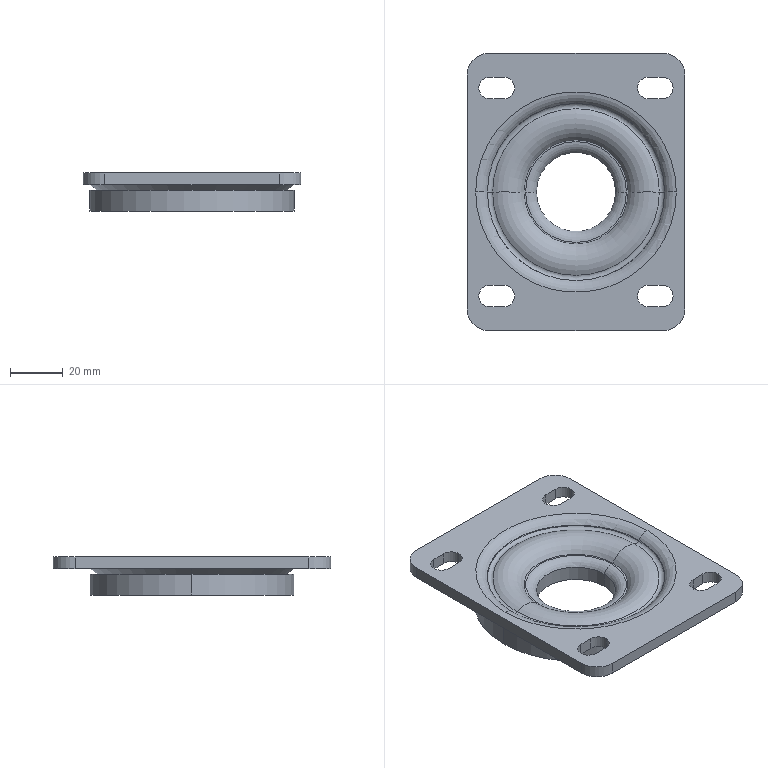Part | SolidWorks | features BaseBody 4, CombineBodies 2, ICE 2, MoveCopyBody 1, MoveFace 1, Scale 1 | 1 solid | 49 faces | box 82.5 x 105 x 14.438 mm | volume 61756 mm3 | cylinder 20 | plane 17 | torus 8 | cone 4 | commonest cylinder face diameters 8.25 x12 16.5 x4 30 x2 77.25 x2
STEP:
#1=CARTESIAN_POINT('',(-15.004,56.345,110.911));
#2=VERTEX_POINT('',#1);
#3=CARTESIAN_POINT('',(14.996,56.345,110.911));
#4=VERTEX_POINT('',#3);
#5=CARTESIAN_POINT('',(-0.004235,56.345,110.911));
#6=DIRECTION('',(0.,0.,1.));
#7=DIRECTION('',(-1.,0.,0.));
#8=AXIS2_PLACEMENT_3D('',#5,#6,#7);
#9=CIRCLE('',#8,15.);
#10=EDGE_CURVE('',#2,#4,#9,.T.);
#11=ORIENTED_EDGE('',*,*,#10,.T.);
#12=CARTESIAN_POINT('',(14.996,56.345,105.247));
#13=VERTEX_POINT('',#12);
#14=CARTESIAN_POINT('',(14.996,56.345,119.684));
#15=DIRECTION('',(0.,0.,-1.));
#16=VECTOR('',#15,1000.);
#17=LINE('',#14,#16);
#18=EDGE_CURVE('',#4,#13,#17,.T.);
#19=ORIENTED_EDGE('',*,*,#18,.T.);
#20=CARTESIAN_POINT('',(-15.004,56.345,105.247));
#21=VERTEX_POINT('',#20);
#22=CARTESIAN_POINT('',(-0.004235,56.345,105.247));
#23=DIRECTION('',(0.,0.,-1.));
#24=DIRECTION('',(-1.,0.,0.));
#25=AXIS2_PLACEMENT_3D('',#22,#23,#24);
#26=CIRCLE('',#25,15.);
#27=EDGE_CURVE('',#13,#21,#26,.T.);
#28=ORIENTED_EDGE('',*,*,#27,.T.);
#29=CARTESIAN_POINT('',(-15.004,56.345,119.684));
#30=DIRECTION('',(0.,0.,-1.));
#31=VECTOR('',#30,1000.);
#32=LINE('',#29,#31);
#33=EDGE_CURVE('',#2,#21,#32,.T.);
#34=ORIENTED_EDGE('',*,*,#33,.F.);
#35=EDGE_LOOP('',(#11,#19,#28,#34));
#36=FACE_OUTER_BOUND('',#35,.T.);
#37=CARTESIAN_POINT('',(-0.004235,56.345,119.684));
#38=DIRECTION('',(0.,0.,-1.));
#39=DIRECTION('',(-1.,0.,0.));
#40=AXIS2_PLACEMENT_3D('',#37,#38,#39);
#41=CYLINDRICAL_SURFACE('',#40,15.);
#42=ADVANCED_FACE('',(#36),#41,.F.);
#43=CARTESIAN_POINT('',(-0.004235,56.345,110.911));
#44=DIRECTION('',(0.,0.,1.));
#45=DIRECTION('',(-1.,0.,0.));
#46=AXIS2_PLACEMENT_3D('',#43,#44,#45);
#47=CIRCLE('',#46,15.);
#48=EDGE_CURVE('',#4,#2,#47,.T.);
#49=ORIENTED_EDGE('',*,*,#48,.F.);
#50=CARTESIAN_POINT('',(19.068,56.345,113.497));
#51=VERTEX_POINT('',#50);
#52=CARTESIAN_POINT('',(19.068,56.345,108.997));
#53=DIRECTION('',(0.,-1.,0.));
#54=DIRECTION('',(0.,0.,-1.));
#55=AXIS2_PLACEMENT_3D('',#52,#53,#54);
#56=CIRCLE('',#55,4.5);
#57=EDGE_CURVE('',#51,#4,#56,.T.);
#58=ORIENTED_EDGE('',*,*,#57,.F.);
#59=CARTESIAN_POINT('',(-19.077,56.345,113.497));
#60=VERTEX_POINT('',#59);
#61=CARTESIAN_POINT('',(-0.004235,56.345,113.497));
#62=DIRECTION('',(0.,0.,1.));
#63=DIRECTION('',(1.,0.,0.));
#64=AXIS2_PLACEMENT_3D('',#61,#62,#63);
#65=CIRCLE('',#64,19.072);
#66=EDGE_CURVE('',#51,#60,#65,.T.);
#67=ORIENTED_EDGE('',*,*,#66,.T.);
#68=CARTESIAN_POINT('',(-19.077,56.345,108.997));
#69=DIRECTION('',(0.,1.,0.));
#70=DIRECTION('',(-1.,0.,0.));
#71=AXIS2_PLACEMENT_3D('',#68,#69,#70);
#72=CIRCLE('',#71,4.5);
#73=EDGE_CURVE('',#60,#2,#72,.T.);
#74=ORIENTED_EDGE('',*,*,#73,.T.);
#75=EDGE_LOOP('',(#49,#58,#67,#74));
#76=FACE_OUTER_BOUND('',#75,.T.);
#77=CARTESIAN_POINT('',(-0.004235,56.345,108.997));
#78=DIRECTION('',(0.,0.,1.));
#79=DIRECTION('',(1.,0.,0.));
#80=AXIS2_PLACEMENT_3D('',#77,#78,#79);
#81=TOROIDAL_SURFACE('',#80,19.072,4.5);
#82=ADVANCED_FACE('',(#76),#81,.T.);
#83=CARTESIAN_POINT('',(31.504,56.345,116.515));
#84=VERTEX_POINT('',#83);
#85=CARTESIAN_POINT('',(-31.512,56.345,116.515));
#86=VERTEX_POINT('',#85);
#87=CARTESIAN_POINT('',(-0.004235,56.345,116.515));
#88=DIRECTION('',(0.,0.,1.));
#89=DIRECTION('',(1.,0.,0.));
#90=AXIS2_PLACEMENT_3D('',#87,#88,#89);
#91=CIRCLE('',#90,31.508);
#92=EDGE_CURVE('',#84,#86,#91,.T.);
#93=ORIENTED_EDGE('',*,*,#92,.T.);
#94=CARTESIAN_POINT('',(-19.74,56.345,113.497));
#95=VERTEX_POINT('',#94);
#96=CARTESIAN_POINT('',(-27.146,56.345,109.077));
#97=DIRECTION('',(0.,1.,0.));
#98=DIRECTION('',(-1.,0.,0.));
#99=AXIS2_PLACEMENT_3D('',#96,#97,#98);
#100=CIRCLE('',#99,8.625);
#101=EDGE_CURVE('',#86,#95,#100,.T.);
#102=ORIENTED_EDGE('',*,*,#101,.T.);
#103=CARTESIAN_POINT('',(19.732,56.345,113.497));
#104=VERTEX_POINT('',#103);
#105=CARTESIAN_POINT('',(-0.004235,56.345,113.497));
#106=DIRECTION('',(0.,0.,1.));
#107=DIRECTION('',(1.,0.,0.));
#108=AXIS2_PLACEMENT_3D('',#105,#106,#107);
#109=CIRCLE('',#108,19.736);
#110=EDGE_CURVE('',#104,#95,#109,.T.);
#111=ORIENTED_EDGE('',*,*,#110,.F.);
#112=CARTESIAN_POINT('',(27.138,56.345,109.077));
#113=DIRECTION('',(0.,-1.,0.));
#114=DIRECTION('',(0.,0.,-1.));
#115=AXIS2_PLACEMENT_3D('',#112,#113,#114);
#116=CIRCLE('',#115,8.625);
#117=EDGE_CURVE('',#84,#104,#116,.T.);
#118=ORIENTED_EDGE('',*,*,#117,.F.);
#119=EDGE_LOOP('',(#93,#102,#111,#118));
#120=FACE_OUTER_BOUND('',#119,.T.);
#121=CARTESIAN_POINT('',(-0.004235,56.345,109.077));
#122=DIRECTION('',(0.,0.,1.));
#123=DIRECTION('',(1.,0.,0.));
#124=AXIS2_PLACEMENT_3D('',#121,#122,#123);
#125=TOROIDAL_SURFACE('',#124,27.142,8.625);
#126=ADVANCED_FACE('',(#120),#125,.T.);
#127=CARTESIAN_POINT('',(-0.004235,56.345,116.515));
#128=DIRECTION('',(0.,0.,1.));
#129=DIRECTION('',(1.,0.,0.));
#130=AXIS2_PLACEMENT_3D('',#127,#128,#129);
#131=CIRCLE('',#130,31.508);
#132=EDGE_CURVE('',#86,#84,#131,.T.);
#133=ORIENTED_EDGE('',*,*,#132,.F.);
#134=CARTESIAN_POINT('',(-33.528,56.345,117.013));
#135=VERTEX_POINT('',#134);
#136=CARTESIAN_POINT('',(-32.261,56.345,117.815));
#137=DIRECTION('',(0.,1.,0.));
#138=DIRECTION('',(-1.,0.,0.));
#139=AXIS2_PLACEMENT_3D('',#136,#137,#138);
#140=CIRCLE('',#139,1.5);
#141=EDGE_CURVE('',#86,#135,#140,.T.);
#142=ORIENTED_EDGE('',*,*,#141,.T.);
#143=CARTESIAN_POINT('',(33.52,56.345,117.013));
#144=VERTEX_POINT('',#143);
#145=CARTESIAN_POINT('',(-0.004235,56.345,117.013));
#146=DIRECTION('',(0.,0.,1.));
#147=DIRECTION('',(1.,0.,0.));
#148=AXIS2_PLACEMENT_3D('',#145,#146,#147);
#149=CIRCLE('',#148,33.524);
#150=EDGE_CURVE('',#135,#144,#149,.T.);
#151=ORIENTED_EDGE('',*,*,#150,.T.);
#152=CARTESIAN_POINT('',(32.252,56.345,117.815));
#153=DIRECTION('',(0.,-1.,0.));
#154=DIRECTION('',(0.,0.,-1.));
#155=AXIS2_PLACEMENT_3D('',#152,#153,#154);
#156=CIRCLE('',#155,1.5);
#157=EDGE_CURVE('',#84,#144,#156,.T.);
#158=ORIENTED_EDGE('',*,*,#157,.F.);
#159=EDGE_LOOP('',(#133,#142,#151,#158));
#160=FACE_OUTER_BOUND('',#159,.T.);
#161=CARTESIAN_POINT('',(-0.004235,56.345,117.815));
#162=DIRECTION('',(0.,0.,1.));
#163=DIRECTION('',(1.,0.,0.));
#164=AXIS2_PLACEMENT_3D('',#161,#162,#163);
#165=TOROIDAL_SURFACE('',#164,32.256,1.5);
#166=ADVANCED_FACE('',(#160),#165,.F.);
#167=ORIENTED_EDGE('',*,*,#150,.F.);
#168=CARTESIAN_POINT('',(-33.673,56.345,117.242));
#169=VERTEX_POINT('',#168);
#170=CARTESIAN_POINT('',(-33.673,56.345,117.242));
#171=DIRECTION('',(-0.5345,0.,0.8452));
#172=VECTOR('',#171,1000.);
#173=LINE('',#170,#172);
#174=EDGE_CURVE('',#135,#169,#173,.T.);
#175=ORIENTED_EDGE('',*,*,#174,.T.);
#176=CARTESIAN_POINT('',(33.665,56.345,117.242));
#177=VERTEX_POINT('',#176);
#178=CARTESIAN_POINT('',(-0.004235,56.345,117.242));
#179=DIRECTION('',(0.,0.,1.));
#180=DIRECTION('',(1.,0.,0.));
#181=AXIS2_PLACEMENT_3D('',#178,#179,#180);
#182=CIRCLE('',#181,33.669);
#183=EDGE_CURVE('',#169,#177,#182,.T.);
#184=ORIENTED_EDGE('',*,*,#183,.T.);
#185=CARTESIAN_POINT('',(33.665,56.345,117.242));
#186=DIRECTION('',(0.5345,0.,0.8452));
#187=VECTOR('',#186,1000.);
#188=LINE('',#185,#187);
#189=EDGE_CURVE('',#144,#177,#188,.T.);
#190=ORIENTED_EDGE('',*,*,#189,.F.);
#191=EDGE_LOOP('',(#167,#175,#184,#190));
#192=FACE_OUTER_BOUND('',#191,.T.);
#193=CARTESIAN_POINT('',(-0.004235,56.345,117.242));
#194=DIRECTION('',(0.,0.,1.));
#195=DIRECTION('',(1.,0.,0.));
#196=AXIS2_PLACEMENT_3D('',#193,#194,#195);
#197=CONICAL_SURFACE('',#196,33.669,0.5639);
#198=ADVANCED_FACE('',(#192),#197,.F.);
#199=CARTESIAN_POINT('',(-37.966,56.345,119.684));
#200=VERTEX_POINT('',#199);
#201=CARTESIAN_POINT('',(37.958,56.345,119.684));
#202=VERTEX_POINT('',#201);
#203=CARTESIAN_POINT('',(-0.004235,56.345,119.684));
#204=DIRECTION('',(0.,0.,-1.));
#205=DIRECTION('',(1.,0.,0.));
#206=AXIS2_PLACEMENT_3D('',#203,#204,#205);
#207=CIRCLE('',#206,37.962);
#208=EDGE_CURVE('',#200,#202,#207,.T.);
#209=ORIENTED_EDGE('',*,*,#208,.F.);
#210=CARTESIAN_POINT('',(-38.11,56.345,114.436));
#211=DIRECTION('',(0.,1.,0.));
#212=DIRECTION('',(-1.,0.,0.));
#213=AXIS2_PLACEMENT_3D('',#210,#211,#212);
#214=CIRCLE('',#213,5.25);
#215=EDGE_CURVE('',#200,#169,#214,.T.);
#216=ORIENTED_EDGE('',*,*,#215,.T.);
#217=CARTESIAN_POINT('',(-0.004235,56.345,117.242));
#218=DIRECTION('',(0.,0.,1.));
#219=DIRECTION('',(1.,0.,0.));
#220=AXIS2_PLACEMENT_3D('',#217,#218,#219);
#221=CIRCLE('',#220,33.669);
#222=EDGE_CURVE('',#177,#169,#221,.T.);
#223=ORIENTED_EDGE('',*,*,#222,.F.);
#224=CARTESIAN_POINT('',(38.102,56.345,114.436));
#225=DIRECTION('',(0.,-1.,0.));
#226=DIRECTION('',(0.,0.,-1.));
#227=AXIS2_PLACEMENT_3D('',#224,#225,#226);
#228=CIRCLE('',#227,5.25);
#229=EDGE_CURVE('',#202,#177,#228,.T.);
#230=ORIENTED_EDGE('',*,*,#229,.F.);
#231=EDGE_LOOP('',(#209,#216,#223,#230));
#232=FACE_OUTER_BOUND('',#231,.T.);
#233=CARTESIAN_POINT('',(-0.004235,56.345,114.436));
#234=DIRECTION('',(0.,0.,1.));
#235=DIRECTION('',(1.,0.,0.));
#236=AXIS2_PLACEMENT_3D('',#233,#234,#235);
#237=TOROIDAL_SURFACE('',#236,38.106,5.25);
#238=ADVANCED_FACE('',(#232),#237,.T.);
#239=CARTESIAN_POINT('',(38.621,56.345,105.247));
#240=VERTEX_POINT('',#239);
#241=CARTESIAN_POINT('',(-38.629,56.345,105.247));
#242=VERTEX_POINT('',#241);
#243=CARTESIAN_POINT('',(-0.004235,56.345,105.247));
#244=DIRECTION('',(0.,0.,1.));
#245=DIRECTION('',(1.,0.,0.));
#246=AXIS2_PLACEMENT_3D('',#243,#244,#245);
#247=CIRCLE('',#246,38.625);
#248=EDGE_CURVE('',#240,#242,#247,.T.);
#249=ORIENTED_EDGE('',*,*,#248,.T.);
#250=CARTESIAN_POINT('',(-38.629,56.345,113.122));
#251=VERTEX_POINT('',#250);
#252=CARTESIAN_POINT('',(-38.629,56.345,2.684));
#253=DIRECTION('',(0.,0.,1.));
#254=VECTOR('',#253,1000.);
#255=LINE('',#252,#254);
#256=EDGE_CURVE('',#242,#251,#255,.T.);
#257=ORIENTED_EDGE('',*,*,#256,.T.);
#258=CARTESIAN_POINT('',(38.621,56.345,113.122));
#259=VERTEX_POINT('',#258);
#260=CARTESIAN_POINT('',(-0.004235,56.345,113.122));
#261=DIRECTION('',(0.,0.,1.));
#262=DIRECTION('',(1.,0.,0.));
#263=AXIS2_PLACEMENT_3D('',#260,#261,#262);
#264=CIRCLE('',#263,38.625);
#265=EDGE_CURVE('',#259,#251,#264,.T.);
#266=ORIENTED_EDGE('',*,*,#265,.F.);
#267=CARTESIAN_POINT('',(38.621,56.345,2.684));
#268=DIRECTION('',(0.,0.,1.));
#269=VECTOR('',#268,1000.);
#270=LINE('',#267,#269);
#271=EDGE_CURVE('',#240,#259,#270,.T.);
#272=ORIENTED_EDGE('',*,*,#271,.F.);
#273=EDGE_LOOP('',(#249,#257,#266,#272));
#274=FACE_OUTER_BOUND('',#273,.T.);
#275=CARTESIAN_POINT('',(-0.004235,56.345,2.684));
#276=DIRECTION('',(0.,0.,1.));
#277=DIRECTION('',(1.,0.,0.));
#278=AXIS2_PLACEMENT_3D('',#275,#276,#277);
#279=CYLINDRICAL_SURFACE('',#278,38.625);
#280=ADVANCED_FACE('',(#274),#279,.T.);
#281=CARTESIAN_POINT('',(35.782,56.345,113.122));
#282=VERTEX_POINT('',#281);
#283=CARTESIAN_POINT('',(-35.79,56.345,113.122));
#284=VERTEX_POINT('',#283);
#285=CARTESIAN_POINT('',(-0.004235,56.345,113.122));
#286=DIRECTION('',(0.,0.,1.));
#287=DIRECTION('',(1.,0.,0.));
#288=AXIS2_PLACEMENT_3D('',#285,#286,#287);
#289=CIRCLE('',#288,35.786);
#290=EDGE_CURVE('',#282,#284,#289,.T.);
#291=ORIENTED_EDGE('',*,*,#290,.T.);
#292=CARTESIAN_POINT('',(-38.629,56.345,115.184));
#293=VERTEX_POINT('',#292);
#294=CARTESIAN_POINT('',(-38.629,56.345,115.184));
#295=DIRECTION('',(-0.809,0.,0.5878));
#296=VECTOR('',#295,1000.);
#297=LINE('',#294,#296);
#298=EDGE_CURVE('',#284,#293,#297,.T.);
#299=ORIENTED_EDGE('',*,*,#298,.T.);
#300=CARTESIAN_POINT('',(38.621,56.345,115.184));
#301=VERTEX_POINT('',#300);
#302=CARTESIAN_POINT('',(-0.004235,56.345,115.184));
#303=DIRECTION('',(0.,0.,-1.));
#304=DIRECTION('',(-1.,0.,0.));
#305=AXIS2_PLACEMENT_3D('',#302,#303,#304);
#306=CIRCLE('',#305,38.625);
#307=EDGE_CURVE('',#293,#301,#306,.T.);
#308=ORIENTED_EDGE('',*,*,#307,.T.);
#309=CARTESIAN_POINT('',(38.621,56.345,115.184));
#310=DIRECTION('',(0.809,0.,0.5878));
#311=VECTOR('',#310,1000.);
#312=LINE('',#309,#311);
#313=EDGE_CURVE('',#282,#301,#312,.T.);
#314=ORIENTED_EDGE('',*,*,#313,.F.);
#315=EDGE_LOOP('',(#291,#299,#308,#314));
#316=FACE_OUTER_BOUND('',#315,.T.);
#317=CARTESIAN_POINT('',(-0.004235,56.345,115.184));
#318=DIRECTION('',(0.,0.,1.));
#319=DIRECTION('',(1.,0.,0.));
#320=AXIS2_PLACEMENT_3D('',#317,#318,#319);
#321=CONICAL_SURFACE('',#320,38.625,0.9425);
#322=ADVANCED_FACE('',(#316),#321,.T.);
#323=CARTESIAN_POINT('',(-27.379,21.095,115.184));
#324=VERTEX_POINT('',#323);
#325=CARTESIAN_POINT('',(-23.254,16.97,115.184));
#326=VERTEX_POINT('',#325);
#327=CARTESIAN_POINT('',(-27.379,16.97,115.184));
#328=DIRECTION('',(0.,0.,-1.));
#329=DIRECTION('',(-1.,0.,0.));
#330=AXIS2_PLACEMENT_3D('',#327,#328,#329);
#331=CIRCLE('',#330,4.125);
#332=EDGE_CURVE('',#324,#326,#331,.T.);
#333=ORIENTED_EDGE('',*,*,#332,.T.);
#334=CARTESIAN_POINT('',(-23.254,16.97,119.684));
#335=VERTEX_POINT('',#334);
#336=CARTESIAN_POINT('',(-23.254,16.97,115.184));
#337=DIRECTION('',(0.,0.,1.));
#338=VECTOR('',#337,1000.);
#339=LINE('',#336,#338);
#340=EDGE_CURVE('',#326,#335,#339,.T.);
#341=ORIENTED_EDGE('',*,*,#340,.T.);
#342=CARTESIAN_POINT('',(-27.379,21.095,119.684));
#343=VERTEX_POINT('',#342);
#344=CARTESIAN_POINT('',(-27.379,16.97,119.684));
#345=DIRECTION('',(0.,0.,-1.));
#346=DIRECTION('',(-1.,0.,0.));
#347=AXIS2_PLACEMENT_3D('',#344,#345,#346);
#348=CIRCLE('',#347,4.125);
#349=EDGE_CURVE('',#343,#335,#348,.T.);
#350=ORIENTED_EDGE('',*,*,#349,.F.);
#351=CARTESIAN_POINT('',(-27.379,21.095,115.184));
#352=DIRECTION('',(0.,0.,1.));
#353=VECTOR('',#352,1000.);
#354=LINE('',#351,#353);
#355=EDGE_CURVE('',#324,#343,#354,.T.);
#356=ORIENTED_EDGE('',*,*,#355,.F.);
#357=EDGE_LOOP('',(#333,#341,#350,#356));
#358=FACE_OUTER_BOUND('',#357,.T.);
#359=CARTESIAN_POINT('',(-27.379,16.97,115.184));
#360=DIRECTION('',(0.,0.,1.));
#361=DIRECTION('',(1.,0.,0.));
#362=AXIS2_PLACEMENT_3D('',#359,#360,#361);
#363=CYLINDRICAL_SURFACE('',#362,4.125);
#364=ADVANCED_FACE('',(#358),#363,.F.);
#365=CARTESIAN_POINT('',(-27.379,99.845,115.184));
#366=VERTEX_POINT('',#365);
#367=CARTESIAN_POINT('',(-23.254,95.72,115.184));
#368=VERTEX_POINT('',#367);
#369=CARTESIAN_POINT('',(-27.379,95.72,115.184));
#370=DIRECTION('',(0.,0.,-1.));
#371=DIRECTION('',(-1.,0.,0.));
#372=AXIS2_PLACEMENT_3D('',#369,#370,#371);
#373=CIRCLE('',#372,4.125);
#374=EDGE_CURVE('',#366,#368,#373,.T.);
#375=ORIENTED_EDGE('',*,*,#374,.T.);
#376=CARTESIAN_POINT('',(-23.254,95.72,119.684));
#377=VERTEX_POINT('',#376);
#378=CARTESIAN_POINT('',(-23.254,95.72,115.184));
#379=DIRECTION('',(0.,0.,1.));
#380=VECTOR('',#379,1000.);
#381=LINE('',#378,#380);
#382=EDGE_CURVE('',#368,#377,#381,.T.);
#383=ORIENTED_EDGE('',*,*,#382,.T.);
#384=CARTESIAN_POINT('',(-27.379,99.845,119.684));
#385=VERTEX_POINT('',#384);
#386=CARTESIAN_POINT('',(-27.379,95.72,119.684));
#387=DIRECTION('',(0.,0.,-1.));
#388=DIRECTION('',(-1.,0.,0.));
#389=AXIS2_PLACEMENT_3D('',#386,#387,#388);
#390=CIRCLE('',#389,4.125);
#391=EDGE_CURVE('',#385,#377,#390,.T.);
#392=ORIENTED_EDGE('',*,*,#391,.F.);
#393=CARTESIAN_POINT('',(-27.379,99.845,115.184));
#394=DIRECTION('',(0.,0.,1.));
#395=VECTOR('',#394,1000.);
#396=LINE('',#393,#395);
#397=EDGE_CURVE('',#366,#385,#396,.T.);
#398=ORIENTED_EDGE('',*,*,#397,.F.);
#399=EDGE_LOOP('',(#375,#383,#392,#398));
#400=FACE_OUTER_BOUND('',#399,.T.);
#401=CARTESIAN_POINT('',(-27.379,95.72,115.184));
#402=DIRECTION('',(0.,0.,1.));
#403=DIRECTION('',(1.,0.,0.));
#404=AXIS2_PLACEMENT_3D('',#401,#402,#403);
#405=CYLINDRICAL_SURFACE('',#404,4.125);
#406=ADVANCED_FACE('',(#400),#405,.F.);
#407=CARTESIAN_POINT('',(32.621,99.845,115.184));
#408=VERTEX_POINT('',#407);
#409=CARTESIAN_POINT('',(36.746,95.72,115.184));
#410=VERTEX_POINT('',#409);
#411=CARTESIAN_POINT('',(32.621,95.72,115.184));
#412=DIRECTION('',(0.,0.,-1.));
#413=DIRECTION('',(-1.,0.,0.));
#414=AXIS2_PLACEMENT_3D('',#411,#412,#413);
#415=CIRCLE('',#414,4.125);
#416=EDGE_CURVE('',#408,#410,#415,.T.);
#417=ORIENTED_EDGE('',*,*,#416,.T.);
#418=CARTESIAN_POINT('',(36.746,95.72,119.684));
#419=VERTEX_POINT('',#418);
#420=CARTESIAN_POINT('',(36.746,95.72,115.184));
#421=DIRECTION('',(0.,0.,1.));
#422=VECTOR('',#421,1000.);
#423=LINE('',#420,#422);
#424=EDGE_CURVE('',#410,#419,#423,.T.);
#425=ORIENTED_EDGE('',*,*,#424,.T.);
#426=CARTESIAN_POINT('',(32.621,99.845,119.684));
#427=VERTEX_POINT('',#426);
#428=CARTESIAN_POINT('',(32.621,95.72,119.684));
#429=DIRECTION('',(0.,0.,-1.));
#430=DIRECTION('',(-1.,0.,0.));
#431=AXIS2_PLACEMENT_3D('',#428,#429,#430);
#432=CIRCLE('',#431,4.125);
#433=EDGE_CURVE('',#427,#419,#432,.T.);
#434=ORIENTED_EDGE('',*,*,#433,.F.);
#435=CARTESIAN_POINT('',(32.621,99.845,115.184));
#436=DIRECTION('',(0.,0.,1.));
#437=VECTOR('',#436,1000.);
#438=LINE('',#435,#437);
#439=EDGE_CURVE('',#408,#427,#438,.T.);
#440=ORIENTED_EDGE('',*,*,#439,.F.);
#441=EDGE_LOOP('',(#417,#425,#434,#440));
#442=FACE_OUTER_BOUND('',#441,.T.);
#443=CARTESIAN_POINT('',(32.621,95.72,115.184));
#444=DIRECTION('',(0.,0.,1.));
#445=DIRECTION('',(1.,0.,0.));
#446=AXIS2_PLACEMENT_3D('',#443,#444,#445);
#447=CYLINDRICAL_SURFACE('',#446,4.125);
#448=ADVANCED_FACE('',(#442),#447,.F.);
#449=CARTESIAN_POINT('',(32.621,21.095,115.184));
#450=VERTEX_POINT('',#449);
#451=CARTESIAN_POINT('',(36.746,16.97,115.184));
#452=VERTEX_POINT('',#451);
#453=CARTESIAN_POINT('',(32.621,16.97,115.184));
#454=DIRECTION('',(0.,0.,-1.));
#455=DIRECTION('',(-1.,0.,0.));
#456=AXIS2_PLACEMENT_3D('',#453,#454,#455);
#457=CIRCLE('',#456,4.125);
#458=EDGE_CURVE('',#450,#452,#457,.T.);
#459=ORIENTED_EDGE('',*,*,#458,.T.);
#460=CARTESIAN_POINT('',(36.746,16.97,119.684));
#461=VERTEX_POINT('',#460);
#462=CARTESIAN_POINT('',(36.746,16.97,115.184));
#463=DIRECTION('',(0.,0.,1.));
#464=VECTOR('',#463,1000.);
#465=LINE('',#462,#464);
#466=EDGE_CURVE('',#452,#461,#465,.T.);
#467=ORIENTED_EDGE('',*,*,#466,.T.);
#468=CARTESIAN_POINT('',(32.621,21.095,119.684));
#469=VERTEX_POINT('',#468);
#470=CARTESIAN_POINT('',(32.621,16.97,119.684));
#471=DIRECTION('',(0.,0.,-1.));
#472=DIRECTION('',(-1.,0.,0.));
#473=AXIS2_PLACEMENT_3D('',#470,#471,#472);
#474=CIRCLE('',#473,4.125);
#475=EDGE_CURVE('',#469,#461,#474,.T.);
#476=ORIENTED_EDGE('',*,*,#475,.F.);
#477=CARTESIAN_POINT('',(32.621,21.095,115.184));
#478=DIRECTION('',(0.,0.,1.));
#479=VECTOR('',#478,1000.);
#480=LINE('',#477,#479);
#481=EDGE_CURVE('',#450,#469,#480,.T.);
#482=ORIENTED_EDGE('',*,*,#481,.F.);
#483=EDGE_LOOP('',(#459,#467,#476,#482));
#484=FACE_OUTER_BOUND('',#483,.T.);
#485=CARTESIAN_POINT('',(32.621,16.97,115.184));
#486=DIRECTION('',(0.,0.,1.));
#487=DIRECTION('',(1.,0.,0.));
#488=AXIS2_PLACEMENT_3D('',#485,#486,#487);
#489=CYLINDRICAL_SURFACE('',#488,4.125);
#490=ADVANCED_FACE('',(#484),#489,.F.);
#491=CARTESIAN_POINT('',(32.996,108.845,119.684));
#492=VERTEX_POINT('',#491);
#493=CARTESIAN_POINT('',(41.246,100.595,119.684));
#494=VERTEX_POINT('',#493);
#495=CARTESIAN_POINT('',(32.996,100.595,119.684));
#496=DIRECTION('',(0.,0.,-1.));
#497=DIRECTION('',(-1.,0.,0.));
#498=AXIS2_PLACEMENT_3D('',#495,#496,#497);
#499=CIRCLE('',#498,8.25);
#500=EDGE_CURVE('',#492,#494,#499,.T.);
#501=ORIENTED_EDGE('',*,*,#500,.T.);
#502=CARTESIAN_POINT('',(41.246,100.595,115.184));
#503=VERTEX_POINT('',#502);
#504=CARTESIAN_POINT('',(41.246,100.595,115.184));
#505=DIRECTION('',(0.,0.,1.));
#506=VECTOR('',#505,1000.);
#507=LINE('',#504,#506);
#508=EDGE_CURVE('',#503,#494,#507,.T.);
#509=ORIENTED_EDGE('',*,*,#508,.F.);
#510=CARTESIAN_POINT('',(32.996,108.845,115.184));
#511=VERTEX_POINT('',#510);
#512=CARTESIAN_POINT('',(32.996,100.595,115.184));
#513=DIRECTION('',(0.,0.,-1.));
#514=DIRECTION('',(-1.,0.,0.));
#515=AXIS2_PLACEMENT_3D('',#512,#513,#514);
#516=CIRCLE('',#515,8.25);
#517=EDGE_CURVE('',#511,#503,#516,.T.);
#518=ORIENTED_EDGE('',*,*,#517,.F.);
#519=CARTESIAN_POINT('',(32.996,108.845,115.184));
#520=DIRECTION('',(0.,0.,1.));
#521=VECTOR('',#520,1000.);
#522=LINE('',#519,#521);
#523=EDGE_CURVE('',#511,#492,#522,.T.);
#524=ORIENTED_EDGE('',*,*,#523,.T.);
#525=EDGE_LOOP('',(#501,#509,#518,#524));
#526=FACE_OUTER_BOUND('',#525,.T.);
#527=CARTESIAN_POINT('',(32.996,100.595,115.184));
#528=DIRECTION('',(0.,0.,1.));
#529=DIRECTION('',(1.,0.,0.));
#530=AXIS2_PLACEMENT_3D('',#527,#528,#529);
#531=CYLINDRICAL_SURFACE('',#530,8.25);
#532=ADVANCED_FACE('',(#526),#531,.T.);
#533=CARTESIAN_POINT('',(41.246,12.095,119.684));
#534=VERTEX_POINT('',#533);
#535=CARTESIAN_POINT('',(41.246,100.595,119.684));
#536=DIRECTION('',(0.,-1.,0.));
#537=VECTOR('',#536,1000.);
#538=LINE('',#535,#537);
#539=EDGE_CURVE('',#494,#534,#538,.T.);
#540=ORIENTED_EDGE('',*,*,#539,.T.);
#541=CARTESIAN_POINT('',(41.246,12.095,115.184));
#542=VERTEX_POINT('',#541);
#543=CARTESIAN_POINT('',(41.246,12.095,115.184));
#544=DIRECTION('',(0.,0.,1.));
#545=VECTOR('',#544,1000.);
#546=LINE('',#543,#545);
#547=EDGE_CURVE('',#542,#534,#546,.T.);
#548=ORIENTED_EDGE('',*,*,#547,.F.);
#549=CARTESIAN_POINT('',(41.246,100.595,115.184));
#550=DIRECTION('',(0.,-1.,0.));
#551=VECTOR('',#550,1000.);
#552=LINE('',#549,#551);
#553=EDGE_CURVE('',#503,#542,#552,.T.);
#554=ORIENTED_EDGE('',*,*,#553,.F.);
#555=ORIENTED_EDGE('',*,*,#508,.T.);
#556=EDGE_LOOP('',(#540,#548,#554,#555));
#557=FACE_OUTER_BOUND('',#556,.T.);
#558=CARTESIAN_POINT('',(41.246,100.595,115.184));
#559=DIRECTION('',(-1.,0.,0.));
#560=DIRECTION('',(0.,1.,0.));
#561=AXIS2_PLACEMENT_3D('',#558,#559,#560);
#562=PLANE('',#561);
#563=ADVANCED_FACE('',(#557),#562,.F.);
#564=CARTESIAN_POINT('',(32.996,3.845,119.684));
#565=VERTEX_POINT('',#564);
#566=CARTESIAN_POINT('',(32.996,12.095,119.684));
#567=DIRECTION('',(0.,0.,-1.));
#568=DIRECTION('',(1.,0.,0.));
#569=AXIS2_PLACEMENT_3D('',#566,#567,#568);
#570=CIRCLE('',#569,8.25);
#571=EDGE_CURVE('',#534,#565,#570,.T.);
#572=ORIENTED_EDGE('',*,*,#571,.T.);
#573=CARTESIAN_POINT('',(32.996,3.845,115.184));
#574=VERTEX_POINT('',#573);
#575=CARTESIAN_POINT('',(32.996,3.845,115.184));
#576=DIRECTION('',(0.,0.,1.));
#577=VECTOR('',#576,1000.);
#578=LINE('',#575,#577);
#579=EDGE_CURVE('',#574,#565,#578,.T.);
#580=ORIENTED_EDGE('',*,*,#579,.F.);
#581=CARTESIAN_POINT('',(32.996,12.095,115.184));
#582=DIRECTION('',(0.,0.,-1.));
#583=DIRECTION('',(1.,0.,0.));
#584=AXIS2_PLACEMENT_3D('',#581,#582,#583);
#585=CIRCLE('',#584,8.25);
#586=EDGE_CURVE('',#542,#574,#585,.T.);
#587=ORIENTED_EDGE('',*,*,#586,.F.);
#588=ORIENTED_EDGE('',*,*,#547,.T.);
#589=EDGE_LOOP('',(#572,#580,#587,#588));
#590=FACE_OUTER_BOUND('',#589,.T.);
#591=CARTESIAN_POINT('',(32.996,12.095,115.184));
#592=DIRECTION('',(0.,0.,1.));
#593=DIRECTION('',(1.,0.,0.));
#594=AXIS2_PLACEMENT_3D('',#591,#592,#593);
#595=CYLINDRICAL_SURFACE('',#594,8.25);
#596=ADVANCED_FACE('',(#590),#595,.T.);
#597=CARTESIAN_POINT('',(-33.004,3.845,119.684));
#598=VERTEX_POINT('',#597);
#599=CARTESIAN_POINT('',(32.996,3.845,119.684));
#600=DIRECTION('',(-1.,0.,0.));
#601=VECTOR('',#600,1000.);
#602=LINE('',#599,#601);
#603=EDGE_CURVE('',#565,#598,#602,.T.);
#604=ORIENTED_EDGE('',*,*,#603,.T.);
#605=CARTESIAN_POINT('',(-33.004,3.845,115.184));
#606=VERTEX_POINT('',#605);
#607=CARTESIAN_POINT('',(-33.004,3.845,115.184));
#608=DIRECTION('',(0.,0.,1.));
#609=VECTOR('',#608,1000.);
#610=LINE('',#607,#609);
#611=EDGE_CURVE('',#606,#598,#610,.T.);
#612=ORIENTED_EDGE('',*,*,#611,.F.);
#613=CARTESIAN_POINT('',(32.996,3.845,115.184));
#614=DIRECTION('',(-1.,0.,0.));
#615=VECTOR('',#614,1000.);
#616=LINE('',#613,#615);
#617=EDGE_CURVE('',#574,#606,#616,.T.);
#618=ORIENTED_EDGE('',*,*,#617,.F.);
#619=ORIENTED_EDGE('',*,*,#579,.T.);
#620=EDGE_LOOP('',(#604,#612,#618,#619));
#621=FACE_OUTER_BOUND('',#620,.T.);
#622=CARTESIAN_POINT('',(32.996,3.845,115.184));
#623=DIRECTION('',(0.,1.,0.));
#624=DIRECTION('',(1.,0.,0.));
#625=AXIS2_PLACEMENT_3D('',#622,#623,#624);
#626=PLANE('',#625);
#627=ADVANCED_FACE('',(#621),#626,.F.);
#628=CARTESIAN_POINT('',(-41.254,12.095,119.684));
#629=VERTEX_POINT('',#628);
#630=CARTESIAN_POINT('',(-33.004,12.095,119.684));
#631=DIRECTION('',(0.,0.,-1.));
#632=DIRECTION('',(1.,0.,0.));
#633=AXIS2_PLACEMENT_3D('',#630,#631,#632);
#634=CIRCLE('',#633,8.25);
#635=EDGE_CURVE('',#598,#629,#634,.T.);
#636=ORIENTED_EDGE('',*,*,#635,.T.);
#637=CARTESIAN_POINT('',(-41.254,12.095,115.184));
#638=VERTEX_POINT('',#637);
#639=CARTESIAN_POINT('',(-41.254,12.095,115.184));
#640=DIRECTION('',(0.,0.,1.));
#641=VECTOR('',#640,1000.);
#642=LINE('',#639,#641);
#643=EDGE_CURVE('',#638,#629,#642,.T.);
#644=ORIENTED_EDGE('',*,*,#643,.F.);
#645=CARTESIAN_POINT('',(-33.004,12.095,115.184));
#646=DIRECTION('',(0.,0.,-1.));
#647=DIRECTION('',(1.,0.,0.));
#648=AXIS2_PLACEMENT_3D('',#645,#646,#647);
#649=CIRCLE('',#648,8.25);
#650=EDGE_CURVE('',#606,#638,#649,.T.);
#651=ORIENTED_EDGE('',*,*,#650,.F.);
#652=ORIENTED_EDGE('',*,*,#611,.T.);
#653=EDGE_LOOP('',(#636,#644,#651,#652));
#654=FACE_OUTER_BOUND('',#653,.T.);
#655=CARTESIAN_POINT('',(-33.004,12.095,115.184));
#656=DIRECTION('',(0.,0.,1.));
#657=DIRECTION('',(1.,0.,0.));
#658=AXIS2_PLACEMENT_3D('',#655,#656,#657);
#659=CYLINDRICAL_SURFACE('',#658,8.25);
#660=ADVANCED_FACE('',(#654),#659,.T.);
#661=CARTESIAN_POINT('',(-41.254,100.595,119.684));
#662=VERTEX_POINT('',#661);
#663=CARTESIAN_POINT('',(-41.254,12.095,119.684));
#664=DIRECTION('',(0.,1.,0.));
#665=VECTOR('',#664,1000.);
#666=LINE('',#663,#665);
#667=EDGE_CURVE('',#629,#662,#666,.T.);
#668=ORIENTED_EDGE('',*,*,#667,.T.);
#669=CARTESIAN_POINT('',(-41.254,100.595,115.184));
#670=VERTEX_POINT('',#669);
#671=CARTESIAN_POINT('',(-41.254,100.595,115.184));
#672=DIRECTION('',(0.,0.,1.));
#673=VECTOR('',#672,1000.);
#674=LINE('',#671,#673);
#675=EDGE_CURVE('',#670,#662,#674,.T.);
#676=ORIENTED_EDGE('',*,*,#675,.F.);
#677=CARTESIAN_POINT('',(-41.254,12.095,115.184));
#678=DIRECTION('',(0.,1.,0.));
#679=VECTOR('',#678,1000.);
#680=LINE('',#677,#679);
#681=EDGE_CURVE('',#638,#670,#680,.T.);
#682=ORIENTED_EDGE('',*,*,#681,.F.);
#683=ORIENTED_EDGE('',*,*,#643,.T.);
#684=EDGE_LOOP('',(#668,#676,#682,#683));
#685=FACE_OUTER_BOUND('',#684,.T.);
#686=CARTESIAN_POINT('',(-41.254,12.095,115.184));
#687=DIRECTION('',(1.,0.,0.));
#688=DIRECTION('',(0.,1.,0.));
#689=AXIS2_PLACEMENT_3D('',#686,#687,#688);
#690=PLANE('',#689);
#691=ADVANCED_FACE('',(#685),#690,.F.);
#692=CARTESIAN_POINT('',(-33.004,108.845,119.684));
#693=VERTEX_POINT('',#692);
#694=CARTESIAN_POINT('',(-33.004,100.595,119.684));
#695=DIRECTION('',(0.,0.,-1.));
#696=DIRECTION('',(1.,0.,0.));
#697=AXIS2_PLACEMENT_3D('',#694,#695,#696);
#698=CIRCLE('',#697,8.25);
#699=EDGE_CURVE('',#662,#693,#698,.T.);
#700=ORIENTED_EDGE('',*,*,#699,.T.);
#701=CARTESIAN_POINT('',(-33.004,108.845,115.184));
#702=VERTEX_POINT('',#701);
#703=CARTESIAN_POINT('',(-33.004,108.845,115.184));
#704=DIRECTION('',(0.,0.,1.));
#705=VECTOR('',#704,1000.);
#706=LINE('',#703,#705);
#707=EDGE_CURVE('',#702,#693,#706,.T.);
#708=ORIENTED_EDGE('',*,*,#707,.F.);
#709=CARTESIAN_POINT('',(-33.004,100.595,115.184));
#710=DIRECTION('',(0.,0.,-1.));
#711=DIRECTION('',(1.,0.,0.));
#712=AXIS2_PLACEMENT_3D('',#709,#710,#711);
#713=CIRCLE('',#712,8.25);
#714=EDGE_CURVE('',#670,#702,#713,.T.);
#715=ORIENTED_EDGE('',*,*,#714,.F.);
#716=ORIENTED_EDGE('',*,*,#675,.T.);
#717=EDGE_LOOP('',(#700,#708,#715,#716));
#718=FACE_OUTER_BOUND('',#717,.T.);
#719=CARTESIAN_POINT('',(-33.004,100.595,115.184));
#720=DIRECTION('',(0.,0.,1.));
#721=DIRECTION('',(1.,0.,0.));
#722=AXIS2_PLACEMENT_3D('',#719,#720,#721);
#723=CYLINDRICAL_SURFACE('',#722,8.25);
#724=ADVANCED_FACE('',(#718),#723,.T.);
#725=CARTESIAN_POINT('',(27.371,99.845,119.684));
#726=VERTEX_POINT('',#725);
#727=CARTESIAN_POINT('',(27.371,99.845,119.684));
#728=DIRECTION('',(1.,0.,0.));
#729=VECTOR('',#728,1000.);
#730=LINE('',#727,#729);
#731=EDGE_CURVE('',#726,#427,#730,.T.);
#732=ORIENTED_EDGE('',*,*,#731,.F.);
#733=CARTESIAN_POINT('',(27.371,99.845,115.184));
#734=VERTEX_POINT('',#733);
#735=CARTESIAN_POINT('',(27.371,99.845,115.184));
#736=DIRECTION('',(0.,0.,1.));
#737=VECTOR('',#736,1000.);
#738=LINE('',#735,#737);
#739=EDGE_CURVE('',#734,#726,#738,.T.);
#740=ORIENTED_EDGE('',*,*,#739,.F.);
#741=CARTESIAN_POINT('',(27.371,99.845,115.184));
#742=DIRECTION('',(1.,0.,0.));
#743=VECTOR('',#742,1000.);
#744=LINE('',#741,#743);
#745=EDGE_CURVE('',#734,#408,#744,.T.);
#746=ORIENTED_EDGE('',*,*,#745,.T.);
#747=ORIENTED_EDGE('',*,*,#439,.T.);
#748=EDGE_LOOP('',(#732,#740,#746,#747));
#749=FACE_OUTER_BOUND('',#748,.T.);
#750=CARTESIAN_POINT('',(27.371,99.845,115.184));
#751=DIRECTION('',(0.,-1.,0.));
#752=DIRECTION('',(0.,0.,-1.));
#753=AXIS2_PLACEMENT_3D('',#750,#751,#752);
#754=PLANE('',#753);
#755=ADVANCED_FACE('',(#749),#754,.T.);
#756=CARTESIAN_POINT('',(27.371,91.595,119.684));
#757=VERTEX_POINT('',#756);
#758=CARTESIAN_POINT('',(27.371,95.72,119.684));
#759=DIRECTION('',(0.,0.,-1.));
#760=DIRECTION('',(1.,0.,0.));
#761=AXIS2_PLACEMENT_3D('',#758,#759,#760);
#762=CIRCLE('',#761,4.125);
#763=EDGE_CURVE('',#757,#726,#762,.T.);
#764=ORIENTED_EDGE('',*,*,#763,.F.);
#765=CARTESIAN_POINT('',(27.371,91.595,115.184));
#766=VERTEX_POINT('',#765);
#767=CARTESIAN_POINT('',(27.371,91.595,115.184));
#768=DIRECTION('',(0.,0.,1.));
#769=VECTOR('',#768,1000.);
#770=LINE('',#767,#769);
#771=EDGE_CURVE('',#766,#757,#770,.T.);
#772=ORIENTED_EDGE('',*,*,#771,.F.);
#773=CARTESIAN_POINT('',(27.371,95.72,115.184));
#774=DIRECTION('',(0.,0.,-1.));
#775=DIRECTION('',(1.,0.,0.));
#776=AXIS2_PLACEMENT_3D('',#773,#774,#775);
#777=CIRCLE('',#776,4.125);
#778=EDGE_CURVE('',#766,#734,#777,.T.);
#779=ORIENTED_EDGE('',*,*,#778,.T.);
#780=ORIENTED_EDGE('',*,*,#739,.T.);
#781=EDGE_LOOP('',(#764,#772,#779,#780));
#782=FACE_OUTER_BOUND('',#781,.T.);
#783=CARTESIAN_POINT('',(27.371,95.72,115.184));
#784=DIRECTION('',(0.,0.,1.));
#785=DIRECTION('',(1.,0.,0.));
#786=AXIS2_PLACEMENT_3D('',#783,#784,#785);
#787=CYLINDRICAL_SURFACE('',#786,4.125);
#788=ADVANCED_FACE('',(#782),#787,.F.);
#789=CARTESIAN_POINT('',(32.621,91.595,119.684));
#790=VERTEX_POINT('',#789);
#791=CARTESIAN_POINT('',(32.621,91.595,119.684));
#792=DIRECTION('',(-1.,0.,0.));
#793=VECTOR('',#792,1000.);
#794=LINE('',#791,#793);
#795=EDGE_CURVE('',#790,#757,#794,.T.);
#796=ORIENTED_EDGE('',*,*,#795,.F.);
#797=CARTESIAN_POINT('',(32.621,91.595,115.184));
#798=VERTEX_POINT('',#797);
#799=CARTESIAN_POINT('',(32.621,91.595,115.184));
#800=DIRECTION('',(0.,0.,1.));
#801=VECTOR('',#800,1000.);
#802=LINE('',#799,#801);
#803=EDGE_CURVE('',#798,#790,#802,.T.);
#804=ORIENTED_EDGE('',*,*,#803,.F.);
#805=CARTESIAN_POINT('',(32.621,91.595,115.184));
#806=DIRECTION('',(-1.,0.,0.));
#807=VECTOR('',#806,1000.);
#808=LINE('',#805,#807);
#809=EDGE_CURVE('',#798,#766,#808,.T.);
#810=ORIENTED_EDGE('',*,*,#809,.T.);
#811=ORIENTED_EDGE('',*,*,#771,.T.);
#812=EDGE_LOOP('',(#796,#804,#810,#811));
#813=FACE_OUTER_BOUND('',#812,.T.);
#814=CARTESIAN_POINT('',(32.621,91.595,115.184));
#815=DIRECTION('',(0.,1.,0.));
#816=DIRECTION('',(1.,0.,0.));
#817=AXIS2_PLACEMENT_3D('',#814,#815,#816);
#818=PLANE('',#817);
#819=ADVANCED_FACE('',(#813),#818,.T.);
#820=CARTESIAN_POINT('',(-32.629,99.845,119.684));
#821=VERTEX_POINT('',#820);
#822=CARTESIAN_POINT('',(-32.629,99.845,119.684));
#823=DIRECTION('',(1.,0.,0.));
#824=VECTOR('',#823,1000.);
#825=LINE('',#822,#824);
#826=EDGE_CURVE('',#821,#385,#825,.T.);
#827=ORIENTED_EDGE('',*,*,#826,.F.);
#828=CARTESIAN_POINT('',(-32.629,99.845,115.184));
#829=VERTEX_POINT('',#828);
#830=CARTESIAN_POINT('',(-32.629,99.845,115.184));
#831=DIRECTION('',(0.,0.,1.));
#832=VECTOR('',#831,1000.);
#833=LINE('',#830,#832);
#834=EDGE_CURVE('',#829,#821,#833,.T.);
#835=ORIENTED_EDGE('',*,*,#834,.F.);
#836=CARTESIAN_POINT('',(-32.629,99.845,115.184));
#837=DIRECTION('',(1.,0.,0.));
#838=VECTOR('',#837,1000.);
#839=LINE('',#836,#838);
#840=EDGE_CURVE('',#829,#366,#839,.T.);
#841=ORIENTED_EDGE('',*,*,#840,.T.);
#842=ORIENTED_EDGE('',*,*,#397,.T.);
#843=EDGE_LOOP('',(#827,#835,#841,#842));
#844=FACE_OUTER_BOUND('',#843,.T.);
#845=CARTESIAN_POINT('',(-32.629,99.845,115.184));
#846=DIRECTION('',(0.,-1.,0.));
#847=DIRECTION('',(0.,0.,-1.));
#848=AXIS2_PLACEMENT_3D('',#845,#846,#847);
#849=PLANE('',#848);
#850=ADVANCED_FACE('',(#844),#849,.T.);
#851=CARTESIAN_POINT('',(-32.629,91.595,119.684));
#852=VERTEX_POINT('',#851);
#853=CARTESIAN_POINT('',(-32.629,95.72,119.684));
#854=DIRECTION('',(0.,0.,-1.));
#855=DIRECTION('',(1.,0.,0.));
#856=AXIS2_PLACEMENT_3D('',#853,#854,#855);
#857=CIRCLE('',#856,4.125);
#858=EDGE_CURVE('',#852,#821,#857,.T.);
#859=ORIENTED_EDGE('',*,*,#858,.F.);
#860=CARTESIAN_POINT('',(-32.629,91.595,115.184));
#861=VERTEX_POINT('',#860);
#862=CARTESIAN_POINT('',(-32.629,91.595,115.184));
#863=DIRECTION('',(0.,0.,1.));
#864=VECTOR('',#863,1000.);
#865=LINE('',#862,#864);
#866=EDGE_CURVE('',#861,#852,#865,.T.);
#867=ORIENTED_EDGE('',*,*,#866,.F.);
#868=CARTESIAN_POINT('',(-32.629,95.72,115.184));
#869=DIRECTION('',(0.,0.,-1.));
#870=DIRECTION('',(1.,0.,0.));
#871=AXIS2_PLACEMENT_3D('',#868,#869,#870);
#872=CIRCLE('',#871,4.125);
#873=EDGE_CURVE('',#861,#829,#872,.T.);
#874=ORIENTED_EDGE('',*,*,#873,.T.);
#875=ORIENTED_EDGE('',*,*,#834,.T.);
#876=EDGE_LOOP('',(#859,#867,#874,#875));
#877=FACE_OUTER_BOUND('',#876,.T.);
#878=CARTESIAN_POINT('',(-32.629,95.72,115.184));
#879=DIRECTION('',(0.,0.,1.));
#880=DIRECTION('',(1.,0.,0.));
#881=AXIS2_PLACEMENT_3D('',#878,#879,#880);
#882=CYLINDRICAL_SURFACE('',#881,4.125);
#883=ADVANCED_FACE('',(#877),#882,.F.);
#884=CARTESIAN_POINT('',(-27.379,91.595,119.684));
#885=VERTEX_POINT('',#884);
#886=CARTESIAN_POINT('',(-27.379,91.595,119.684));
#887=DIRECTION('',(-1.,0.,0.));
#888=VECTOR('',#887,1000.);
#889=LINE('',#886,#888);
#890=EDGE_CURVE('',#885,#852,#889,.T.);
#891=ORIENTED_EDGE('',*,*,#890,.F.);
#892=CARTESIAN_POINT('',(-27.379,91.595,115.184));
#893=VERTEX_POINT('',#892);
#894=CARTESIAN_POINT('',(-27.379,91.595,115.184));
#895=DIRECTION('',(0.,0.,1.));
#896=VECTOR('',#895,1000.);
#897=LINE('',#894,#896);
#898=EDGE_CURVE('',#893,#885,#897,.T.);
#899=ORIENTED_EDGE('',*,*,#898,.F.);
#900=CARTESIAN_POINT('',(-27.379,91.595,115.184));
#901=DIRECTION('',(-1.,0.,0.));
#902=VECTOR('',#901,1000.);
#903=LINE('',#900,#902);
#904=EDGE_CURVE('',#893,#861,#903,.T.);
#905=ORIENTED_EDGE('',*,*,#904,.T.);
#906=ORIENTED_EDGE('',*,*,#866,.T.);
#907=EDGE_LOOP('',(#891,#899,#905,#906));
#908=FACE_OUTER_BOUND('',#907,.T.);
#909=CARTESIAN_POINT('',(-27.379,91.595,115.184));
#910=DIRECTION('',(0.,1.,0.));
#911=DIRECTION('',(1.,0.,0.));
#912=AXIS2_PLACEMENT_3D('',#909,#910,#911);
#913=PLANE('',#912);
#914=ADVANCED_FACE('',(#908),#913,.T.);
#915=CARTESIAN_POINT('',(-32.629,21.095,119.684));
#916=VERTEX_POINT('',#915);
#917=CARTESIAN_POINT('',(-32.629,21.095,119.684));
#918=DIRECTION('',(1.,0.,0.));
#919=VECTOR('',#918,1000.);
#920=LINE('',#917,#919);
#921=EDGE_CURVE('',#916,#343,#920,.T.);
#922=ORIENTED_EDGE('',*,*,#921,.F.);
#923=CARTESIAN_POINT('',(-32.629,21.095,115.184));
#924=VERTEX_POINT('',#923);
#925=CARTESIAN_POINT('',(-32.629,21.095,115.184));
#926=DIRECTION('',(0.,0.,1.));
#927=VECTOR('',#926,1000.);
#928=LINE('',#925,#927);
#929=EDGE_CURVE('',#924,#916,#928,.T.);
#930=ORIENTED_EDGE('',*,*,#929,.F.);
#931=CARTESIAN_POINT('',(-32.629,21.095,115.184));
#932=DIRECTION('',(1.,0.,0.));
#933=VECTOR('',#932,1000.);
#934=LINE('',#931,#933);
#935=EDGE_CURVE('',#924,#324,#934,.T.);
#936=ORIENTED_EDGE('',*,*,#935,.T.);
#937=ORIENTED_EDGE('',*,*,#355,.T.);
#938=EDGE_LOOP('',(#922,#930,#936,#937));
#939=FACE_OUTER_BOUND('',#938,.T.);
#940=CARTESIAN_POINT('',(-32.629,21.095,115.184));
#941=DIRECTION('',(0.,-1.,0.));
#942=DIRECTION('',(-1.,0.,0.));
#943=AXIS2_PLACEMENT_3D('',#940,#941,#942);
#944=PLANE('',#943);
#945=ADVANCED_FACE('',(#939),#944,.T.);
#946=CARTESIAN_POINT('',(-32.629,12.845,119.684));
#947=VERTEX_POINT('',#946);
#948=CARTESIAN_POINT('',(-32.629,16.97,119.684));
#949=DIRECTION('',(0.,0.,-1.));
#950=DIRECTION('',(1.,0.,0.));
#951=AXIS2_PLACEMENT_3D('',#948,#949,#950);
#952=CIRCLE('',#951,4.125);
#953=EDGE_CURVE('',#947,#916,#952,.T.);
#954=ORIENTED_EDGE('',*,*,#953,.F.);
#955=CARTESIAN_POINT('',(-32.629,12.845,115.184));
#956=VERTEX_POINT('',#955);
#957=CARTESIAN_POINT('',(-32.629,12.845,115.184));
#958=DIRECTION('',(0.,0.,1.));
#959=VECTOR('',#958,1000.);
#960=LINE('',#957,#959);
#961=EDGE_CURVE('',#956,#947,#960,.T.);
#962=ORIENTED_EDGE('',*,*,#961,.F.);
#963=CARTESIAN_POINT('',(-32.629,16.97,115.184));
#964=DIRECTION('',(0.,0.,-1.));
#965=DIRECTION('',(1.,0.,0.));
#966=AXIS2_PLACEMENT_3D('',#963,#964,#965);
#967=CIRCLE('',#966,4.125);
#968=EDGE_CURVE('',#956,#924,#967,.T.);
#969=ORIENTED_EDGE('',*,*,#968,.T.);
#970=ORIENTED_EDGE('',*,*,#929,.T.);
#971=EDGE_LOOP('',(#954,#962,#969,#970));
#972=FACE_OUTER_BOUND('',#971,.T.);
#973=CARTESIAN_POINT('',(-32.629,16.97,115.184));
#974=DIRECTION('',(0.,0.,1.));
#975=DIRECTION('',(1.,0.,0.));
#976=AXIS2_PLACEMENT_3D('',#973,#974,#975);
#977=CYLINDRICAL_SURFACE('',#976,4.125);
#978=ADVANCED_FACE('',(#972),#977,.F.);
#979=CARTESIAN_POINT('',(-27.379,12.845,119.684));
#980=VERTEX_POINT('',#979);
#981=CARTESIAN_POINT('',(-27.379,12.845,119.684));
#982=DIRECTION('',(-1.,0.,0.));
#983=VECTOR('',#982,1000.);
#984=LINE('',#981,#983);
#985=EDGE_CURVE('',#980,#947,#984,.T.);
#986=ORIENTED_EDGE('',*,*,#985,.F.);
#987=CARTESIAN_POINT('',(-27.379,12.845,115.184));
#988=VERTEX_POINT('',#987);
#989=CARTESIAN_POINT('',(-27.379,12.845,115.184));
#990=DIRECTION('',(0.,0.,1.));
#991=VECTOR('',#990,1000.);
#992=LINE('',#989,#991);
#993=EDGE_CURVE('',#988,#980,#992,.T.);
#994=ORIENTED_EDGE('',*,*,#993,.F.);
#995=CARTESIAN_POINT('',(-27.379,12.845,115.184));
#996=DIRECTION('',(-1.,0.,0.));
#997=VECTOR('',#996,1000.);
#998=LINE('',#995,#997);
#999=EDGE_CURVE('',#988,#956,#998,.T.);
#1000=ORIENTED_EDGE('',*,*,#999,.T.);
#1001=ORIENTED_EDGE('',*,*,#961,.T.);
#1002=EDGE_LOOP('',(#986,#994,#1000,#1001));
#1003=FACE_OUTER_BOUND('',#1002,.T.);
#1004=CARTESIAN_POINT('',(-27.379,12.845,115.184));
#1005=DIRECTION('',(0.,1.,0.));
#1006=DIRECTION('',(1.,0.,0.));
#1007=AXIS2_PLACEMENT_3D('',#1004,#1005,#1006);
#1008=PLANE('',#1007);
#1009=ADVANCED_FACE('',(#1003),#1008,.T.);
#1010=CARTESIAN_POINT('',(27.371,12.845,119.684));
#1011=VERTEX_POINT('',#1010);
#1012=CARTESIAN_POINT('',(27.371,21.095,119.684));
#1013=VERTEX_POINT('',#1012);
#1014=CARTESIAN_POINT('',(27.371,16.97,119.684));
#1015=DIRECTION('',(0.,0.,-1.));
#1016=DIRECTION('',(1.,0.,0.));
#1017=AXIS2_PLACEMENT_3D('',#1014,#1015,#1016);
#1018=CIRCLE('',#1017,4.125);
#1019=EDGE_CURVE('',#1011,#1013,#1018,.T.);
#1020=ORIENTED_EDGE('',*,*,#1019,.F.);
#1021=CARTESIAN_POINT('',(27.371,12.845,115.184));
#1022=VERTEX_POINT('',#1021);
#1023=CARTESIAN_POINT('',(27.371,12.845,115.184));
#1024=DIRECTION('',(0.,0.,1.));
#1025=VECTOR('',#1024,1000.);
#1026=LINE('',#1023,#1025);
#1027=EDGE_CURVE('',#1022,#1011,#1026,.T.);
#1028=ORIENTED_EDGE('',*,*,#1027,.F.);
#1029=CARTESIAN_POINT('',(27.371,21.095,115.184));
#1030=VERTEX_POINT('',#1029);
#1031=CARTESIAN_POINT('',(27.371,16.97,115.184));
#1032=DIRECTION('',(0.,0.,-1.));
#1033=DIRECTION('',(1.,0.,0.));
#1034=AXIS2_PLACEMENT_3D('',#1031,#1032,#1033);
#1035=CIRCLE('',#1034,4.125);
#1036=EDGE_CURVE('',#1022,#1030,#1035,.T.);
#1037=ORIENTED_EDGE('',*,*,#1036,.T.);
#1038=CARTESIAN_POINT('',(27.371,21.095,115.184));
#1039=DIRECTION('',(0.,0.,1.));
#1040=VECTOR('',#1039,1000.);
#1041=LINE('',#1038,#1040);
#1042=EDGE_CURVE('',#1030,#1013,#1041,.T.);
#1043=ORIENTED_EDGE('',*,*,#1042,.T.);
#1044=EDGE_LOOP('',(#1020,#1028,#1037,#1043));
#1045=FACE_OUTER_BOUND('',#1044,.T.);
#1046=CARTESIAN_POINT('',(27.371,16.97,115.184));
#1047=DIRECTION('',(0.,0.,1.));
#1048=DIRECTION('',(1.,0.,0.));
#1049=AXIS2_PLACEMENT_3D('',#1046,#1047,#1048);
#1050=CYLINDRICAL_SURFACE('',#1049,4.125);
#1051=ADVANCED_FACE('',(#1045),#1050,.F.);
#1052=CARTESIAN_POINT('',(32.621,12.845,119.684));
#1053=VERTEX_POINT('',#1052);
#1054=CARTESIAN_POINT('',(32.621,12.845,119.684));
#1055=DIRECTION('',(-1.,0.,0.));
#1056=VECTOR('',#1055,1000.);
#1057=LINE('',#1054,#1056);
#1058=EDGE_CURVE('',#1053,#1011,#1057,.T.);
#1059=ORIENTED_EDGE('',*,*,#1058,.F.);
#1060=CARTESIAN_POINT('',(32.621,12.845,115.184));
#1061=VERTEX_POINT('',#1060);
#1062=CARTESIAN_POINT('',(32.621,12.845,115.184));
#1063=DIRECTION('',(0.,0.,1.));
#1064=VECTOR('',#1063,1000.);
#1065=LINE('',#1062,#1064);
#1066=EDGE_CURVE('',#1061,#1053,#1065,.T.);
#1067=ORIENTED_EDGE('',*,*,#1066,.F.);
#1068=CARTESIAN_POINT('',(32.621,12.845,115.184));
#1069=DIRECTION('',(-1.,0.,0.));
#1070=VECTOR('',#1069,1000.);
#1071=LINE('',#1068,#1070);
#1072=EDGE_CURVE('',#1061,#1022,#1071,.T.);
#1073=ORIENTED_EDGE('',*,*,#1072,.T.);
#1074=ORIENTED_EDGE('',*,*,#1027,.T.);
#1075=EDGE_LOOP('',(#1059,#1067,#1073,#1074));
#1076=FACE_OUTER_BOUND('',#1075,.T.);
#1077=CARTESIAN_POINT('',(32.621,12.845,115.184));
#1078=DIRECTION('',(0.,1.,0.));
#1079=DIRECTION('',(1.,0.,0.));
#1080=AXIS2_PLACEMENT_3D('',#1077,#1078,#1079);
#1081=PLANE('',#1080);
#1082=ADVANCED_FACE('',(#1076),#1081,.T.);
#1083=ORIENTED_EDGE('',*,*,#466,.F.);
#1084=CARTESIAN_POINT('',(32.621,16.97,115.184));
#1085=DIRECTION('',(0.,0.,-1.));
#1086=DIRECTION('',(-1.,0.,0.));
#1087=AXIS2_PLACEMENT_3D('',#1084,#1085,#1086);
#1088=CIRCLE('',#1087,4.125);
#1089=EDGE_CURVE('',#452,#1061,#1088,.T.);
#1090=ORIENTED_EDGE('',*,*,#1089,.T.);
#1091=ORIENTED_EDGE('',*,*,#1066,.T.);
#1092=CARTESIAN_POINT('',(32.621,16.97,119.684));
#1093=DIRECTION('',(0.,0.,-1.));
#1094=DIRECTION('',(-1.,0.,0.));
#1095=AXIS2_PLACEMENT_3D('',#1092,#1093,#1094);
#1096=CIRCLE('',#1095,4.125);
#1097=EDGE_CURVE('',#461,#1053,#1096,.T.);
#1098=ORIENTED_EDGE('',*,*,#1097,.F.);
#1099=EDGE_LOOP('',(#1083,#1090,#1091,#1098));
#1100=FACE_OUTER_BOUND('',#1099,.T.);
#1101=CARTESIAN_POINT('',(32.621,16.97,115.184));
#1102=DIRECTION('',(0.,0.,1.));
#1103=DIRECTION('',(1.,0.,0.));
#1104=AXIS2_PLACEMENT_3D('',#1101,#1102,#1103);
#1105=CYLINDRICAL_SURFACE('',#1104,4.125);
#1106=ADVANCED_FACE('',(#1100),#1105,.F.);
#1107=ORIENTED_EDGE('',*,*,#424,.F.);
#1108=CARTESIAN_POINT('',(32.621,95.72,115.184));
#1109=DIRECTION('',(0.,0.,-1.));
#1110=DIRECTION('',(-1.,0.,0.));
#1111=AXIS2_PLACEMENT_3D('',#1108,#1109,#1110);
#1112=CIRCLE('',#1111,4.125);
#1113=EDGE_CURVE('',#410,#798,#1112,.T.);
#1114=ORIENTED_EDGE('',*,*,#1113,.T.);
#1115=ORIENTED_EDGE('',*,*,#803,.T.);
#1116=CARTESIAN_POINT('',(32.621,95.72,119.684));
#1117=DIRECTION('',(0.,0.,-1.));
#1118=DIRECTION('',(-1.,0.,0.));
#1119=AXIS2_PLACEMENT_3D('',#1116,#1117,#1118);
#1120=CIRCLE('',#1119,4.125);
#1121=EDGE_CURVE('',#419,#790,#1120,.T.);
#1122=ORIENTED_EDGE('',*,*,#1121,.F.);
#1123=EDGE_LOOP('',(#1107,#1114,#1115,#1122));
#1124=FACE_OUTER_BOUND('',#1123,.T.);
#1125=CARTESIAN_POINT('',(32.621,95.72,115.184));
#1126=DIRECTION('',(0.,0.,1.));
#1127=DIRECTION('',(1.,0.,0.));
#1128=AXIS2_PLACEMENT_3D('',#1125,#1126,#1127);
#1129=CYLINDRICAL_SURFACE('',#1128,4.125);
#1130=ADVANCED_FACE('',(#1124),#1129,.F.);
#1131=ORIENTED_EDGE('',*,*,#382,.F.);
#1132=CARTESIAN_POINT('',(-27.379,95.72,115.184));
#1133=DIRECTION('',(0.,0.,-1.));
#1134=DIRECTION('',(-1.,0.,0.));
#1135=AXIS2_PLACEMENT_3D('',#1132,#1133,#1134);
#1136=CIRCLE('',#1135,4.125);
#1137=EDGE_CURVE('',#368,#893,#1136,.T.);
#1138=ORIENTED_EDGE('',*,*,#1137,.T.);
#1139=ORIENTED_EDGE('',*,*,#898,.T.);
#1140=CARTESIAN_POINT('',(-27.379,95.72,119.684));
#1141=DIRECTION('',(0.,0.,-1.));
#1142=DIRECTION('',(-1.,0.,0.));
#1143=AXIS2_PLACEMENT_3D('',#1140,#1141,#1142);
#1144=CIRCLE('',#1143,4.125);
#1145=EDGE_CURVE('',#377,#885,#1144,.T.);
#1146=ORIENTED_EDGE('',*,*,#1145,.F.);
#1147=EDGE_LOOP('',(#1131,#1138,#1139,#1146));
#1148=FACE_OUTER_BOUND('',#1147,.T.);
#1149=CARTESIAN_POINT('',(-27.379,95.72,115.184));
#1150=DIRECTION('',(0.,0.,1.));
#1151=DIRECTION('',(1.,0.,0.));
#1152=AXIS2_PLACEMENT_3D('',#1149,#1150,#1151);
#1153=CYLINDRICAL_SURFACE('',#1152,4.125);
#1154=ADVANCED_FACE('',(#1148),#1153,.F.);
#1155=ORIENTED_EDGE('',*,*,#340,.F.);
#1156=CARTESIAN_POINT('',(-27.379,16.97,115.184));
#1157=DIRECTION('',(0.,0.,-1.));
#1158=DIRECTION('',(-1.,0.,0.));
#1159=AXIS2_PLACEMENT_3D('',#1156,#1157,#1158);
#1160=CIRCLE('',#1159,4.125);
#1161=EDGE_CURVE('',#326,#988,#1160,.T.);
#1162=ORIENTED_EDGE('',*,*,#1161,.T.);
#1163=ORIENTED_EDGE('',*,*,#993,.T.);
#1164=CARTESIAN_POINT('',(-27.379,16.97,119.684));
#1165=DIRECTION('',(0.,0.,-1.));
#1166=DIRECTION('',(-1.,0.,0.));
#1167=AXIS2_PLACEMENT_3D('',#1164,#1165,#1166);
#1168=CIRCLE('',#1167,4.125);
#1169=EDGE_CURVE('',#335,#980,#1168,.T.);
#1170=ORIENTED_EDGE('',*,*,#1169,.F.);
#1171=EDGE_LOOP('',(#1155,#1162,#1163,#1170));
#1172=FACE_OUTER_BOUND('',#1171,.T.);
#1173=CARTESIAN_POINT('',(-27.379,16.97,115.184));
#1174=DIRECTION('',(0.,0.,1.));
#1175=DIRECTION('',(1.,0.,0.));
#1176=AXIS2_PLACEMENT_3D('',#1173,#1174,#1175);
#1177=CYLINDRICAL_SURFACE('',#1176,4.125);
#1178=ADVANCED_FACE('',(#1172),#1177,.F.);
#1179=CARTESIAN_POINT('',(27.371,21.095,119.684));
#1180=DIRECTION('',(1.,0.,0.));
#1181=VECTOR('',#1180,1000.);
#1182=LINE('',#1179,#1181);
#1183=EDGE_CURVE('',#1013,#469,#1182,.T.);
#1184=ORIENTED_EDGE('',*,*,#1183,.F.);
#1185=ORIENTED_EDGE('',*,*,#1042,.F.);
#1186=CARTESIAN_POINT('',(27.371,21.095,115.184));
#1187=DIRECTION('',(1.,0.,0.));
#1188=VECTOR('',#1187,1000.);
#1189=LINE('',#1186,#1188);
#1190=EDGE_CURVE('',#1030,#450,#1189,.T.);
#1191=ORIENTED_EDGE('',*,*,#1190,.T.);
#1192=ORIENTED_EDGE('',*,*,#481,.T.);
#1193=EDGE_LOOP('',(#1184,#1185,#1191,#1192));
#1194=FACE_OUTER_BOUND('',#1193,.T.);
#1195=CARTESIAN_POINT('',(27.371,21.095,115.184));
#1196=DIRECTION('',(0.,-1.,0.));
#1197=DIRECTION('',(0.,0.,-1.));
#1198=AXIS2_PLACEMENT_3D('',#1195,#1196,#1197);
#1199=PLANE('',#1198);
#1200=ADVANCED_FACE('',(#1194),#1199,.T.);
#1201=CARTESIAN_POINT('',(-33.004,108.845,119.684));
#1202=DIRECTION('',(1.,0.,0.));
#1203=VECTOR('',#1202,1000.);
#1204=LINE('',#1201,#1203);
#1205=EDGE_CURVE('',#693,#492,#1204,.T.);
#1206=ORIENTED_EDGE('',*,*,#1205,.T.);
#1207=ORIENTED_EDGE('',*,*,#523,.F.);
#1208=CARTESIAN_POINT('',(-33.004,108.845,115.184));
#1209=DIRECTION('',(1.,0.,0.));
#1210=VECTOR('',#1209,1000.);
#1211=LINE('',#1208,#1210);
#1212=EDGE_CURVE('',#702,#511,#1211,.T.);
#1213=ORIENTED_EDGE('',*,*,#1212,.F.);
#1214=ORIENTED_EDGE('',*,*,#707,.T.);
#1215=EDGE_LOOP('',(#1206,#1207,#1213,#1214));
#1216=FACE_OUTER_BOUND('',#1215,.T.);
#1217=CARTESIAN_POINT('',(-33.004,108.845,115.184));
#1218=DIRECTION('',(0.,-1.,0.));
#1219=DIRECTION('',(0.,0.,-1.));
#1220=AXIS2_PLACEMENT_3D('',#1217,#1218,#1219);
#1221=PLANE('',#1220);
#1222=ADVANCED_FACE('',(#1216),#1221,.F.);
#1223=ORIENTED_EDGE('',*,*,#517,.T.);
#1224=ORIENTED_EDGE('',*,*,#553,.T.);
#1225=ORIENTED_EDGE('',*,*,#586,.T.);
#1226=ORIENTED_EDGE('',*,*,#617,.T.);
#1227=ORIENTED_EDGE('',*,*,#650,.T.);
#1228=ORIENTED_EDGE('',*,*,#681,.T.);
#1229=ORIENTED_EDGE('',*,*,#714,.T.);
#1230=ORIENTED_EDGE('',*,*,#1212,.T.);
#1231=EDGE_LOOP('',(#1223,#1224,#1225,#1226,#1227,#1228,#1229,#1230));
#1232=FACE_OUTER_BOUND('',#1231,.T.);
#1233=CARTESIAN_POINT('',(-0.004235,56.345,115.184));
#1234=DIRECTION('',(0.,0.,-1.));
#1235=DIRECTION('',(-1.,0.,0.));
#1236=AXIS2_PLACEMENT_3D('',#1233,#1234,#1235);
#1237=CIRCLE('',#1236,38.625);
#1238=EDGE_CURVE('',#301,#293,#1237,.T.);
#1239=ORIENTED_EDGE('',*,*,#1238,.F.);
#1240=ORIENTED_EDGE('',*,*,#307,.F.);
#1241=EDGE_LOOP('',(#1239,#1240));
#1242=FACE_BOUND('',#1241,.T.);
#1243=ORIENTED_EDGE('',*,*,#1036,.F.);
#1244=ORIENTED_EDGE('',*,*,#1072,.F.);
#1245=ORIENTED_EDGE('',*,*,#1089,.F.);
#1246=ORIENTED_EDGE('',*,*,#458,.F.);
#1247=ORIENTED_EDGE('',*,*,#1190,.F.);
#1248=EDGE_LOOP('',(#1243,#1244,#1245,#1246,#1247));
#1249=FACE_BOUND('',#1248,.T.);
#1250=ORIENTED_EDGE('',*,*,#935,.F.);
#1251=ORIENTED_EDGE('',*,*,#968,.F.);
#1252=ORIENTED_EDGE('',*,*,#999,.F.);
#1253=ORIENTED_EDGE('',*,*,#1161,.F.);
#1254=ORIENTED_EDGE('',*,*,#332,.F.);
#1255=EDGE_LOOP('',(#1250,#1251,#1252,#1253,#1254));
#1256=FACE_BOUND('',#1255,.T.);
#1257=ORIENTED_EDGE('',*,*,#840,.F.);
#1258=ORIENTED_EDGE('',*,*,#873,.F.);
#1259=ORIENTED_EDGE('',*,*,#904,.F.);
#1260=ORIENTED_EDGE('',*,*,#1137,.F.);
#1261=ORIENTED_EDGE('',*,*,#374,.F.);
#1262=EDGE_LOOP('',(#1257,#1258,#1259,#1260,#1261));
#1263=FACE_BOUND('',#1262,.T.);
#1264=ORIENTED_EDGE('',*,*,#745,.F.);
#1265=ORIENTED_EDGE('',*,*,#778,.F.);
#1266=ORIENTED_EDGE('',*,*,#809,.F.);
#1267=ORIENTED_EDGE('',*,*,#1113,.F.);
#1268=ORIENTED_EDGE('',*,*,#416,.F.);
#1269=EDGE_LOOP('',(#1264,#1265,#1266,#1267,#1268));
#1270=FACE_BOUND('',#1269,.T.);
#1271=CARTESIAN_POINT('',(32.996,100.595,115.184));
#1272=DIRECTION('',(0.,0.,-1.));
#1273=DIRECTION('',(0.,-1.,0.));
#1274=AXIS2_PLACEMENT_3D('',#1271,#1272,#1273);
#1275=PLANE('',#1274);
#1276=ADVANCED_FACE('',(#1232,#1242,#1249,#1256,#1263,#1270),#1275,.T.);
#1277=ORIENTED_EDGE('',*,*,#500,.F.);
#1278=ORIENTED_EDGE('',*,*,#1205,.F.);
#1279=ORIENTED_EDGE('',*,*,#699,.F.);
#1280=ORIENTED_EDGE('',*,*,#667,.F.);
#1281=ORIENTED_EDGE('',*,*,#635,.F.);
#1282=ORIENTED_EDGE('',*,*,#603,.F.);
#1283=ORIENTED_EDGE('',*,*,#571,.F.);
#1284=ORIENTED_EDGE('',*,*,#539,.F.);
#1285=EDGE_LOOP('',(#1277,#1278,#1279,#1280,#1281,#1282,#1283,#1284));
#1286=FACE_OUTER_BOUND('',#1285,.T.);
#1287=CARTESIAN_POINT('',(-0.004235,56.345,119.684));
#1288=DIRECTION('',(0.,0.,-1.));
#1289=DIRECTION('',(1.,0.,0.));
#1290=AXIS2_PLACEMENT_3D('',#1287,#1288,#1289);
#1291=CIRCLE('',#1290,37.962);
#1292=EDGE_CURVE('',#202,#200,#1291,.T.);
#1293=ORIENTED_EDGE('',*,*,#1292,.T.);
#1294=ORIENTED_EDGE('',*,*,#208,.T.);
#1295=EDGE_LOOP('',(#1293,#1294));
#1296=FACE_BOUND('',#1295,.T.);
#1297=ORIENTED_EDGE('',*,*,#731,.T.);
#1298=ORIENTED_EDGE('',*,*,#433,.T.);
#1299=ORIENTED_EDGE('',*,*,#1121,.T.);
#1300=ORIENTED_EDGE('',*,*,#795,.T.);
#1301=ORIENTED_EDGE('',*,*,#763,.T.);
#1302=EDGE_LOOP('',(#1297,#1298,#1299,#1300,#1301));
#1303=FACE_BOUND('',#1302,.T.);
#1304=ORIENTED_EDGE('',*,*,#826,.T.);
#1305=ORIENTED_EDGE('',*,*,#391,.T.);
#1306=ORIENTED_EDGE('',*,*,#1145,.T.);
#1307=ORIENTED_EDGE('',*,*,#890,.T.);
#1308=ORIENTED_EDGE('',*,*,#858,.T.);
#1309=EDGE_LOOP('',(#1304,#1305,#1306,#1307,#1308));
#1310=FACE_BOUND('',#1309,.T.);
#1311=ORIENTED_EDGE('',*,*,#921,.T.);
#1312=ORIENTED_EDGE('',*,*,#349,.T.);
#1313=ORIENTED_EDGE('',*,*,#1169,.T.);
#1314=ORIENTED_EDGE('',*,*,#985,.T.);
#1315=ORIENTED_EDGE('',*,*,#953,.T.);
#1316=EDGE_LOOP('',(#1311,#1312,#1313,#1314,#1315));
#1317=FACE_BOUND('',#1316,.T.);
#1318=ORIENTED_EDGE('',*,*,#1019,.T.);
#1319=ORIENTED_EDGE('',*,*,#1183,.T.);
#1320=ORIENTED_EDGE('',*,*,#475,.T.);
#1321=ORIENTED_EDGE('',*,*,#1097,.T.);
#1322=ORIENTED_EDGE('',*,*,#1058,.T.);
#1323=EDGE_LOOP('',(#1318,#1319,#1320,#1321,#1322));
#1324=FACE_BOUND('',#1323,.T.);
#1325=CARTESIAN_POINT('',(32.996,100.595,119.684));
#1326=DIRECTION('',(0.,0.,-1.));
#1327=DIRECTION('',(0.,-1.,0.));
#1328=AXIS2_PLACEMENT_3D('',#1325,#1326,#1327);
#1329=PLANE('',#1328);
#1330=ADVANCED_FACE('',(#1286,#1296,#1303,#1310,#1317,#1324),#1329,.F.);
#1331=ORIENTED_EDGE('',*,*,#298,.F.);
#1332=CARTESIAN_POINT('',(-0.004235,56.345,113.122));
#1333=DIRECTION('',(0.,0.,1.));
#1334=DIRECTION('',(1.,0.,0.));
#1335=AXIS2_PLACEMENT_3D('',#1332,#1333,#1334);
#1336=CIRCLE('',#1335,35.786);
#1337=EDGE_CURVE('',#284,#282,#1336,.T.);
#1338=ORIENTED_EDGE('',*,*,#1337,.T.);
#1339=ORIENTED_EDGE('',*,*,#313,.T.);
#1340=ORIENTED_EDGE('',*,*,#1238,.T.);
#1341=EDGE_LOOP('',(#1331,#1338,#1339,#1340));
#1342=FACE_OUTER_BOUND('',#1341,.T.);
#1343=CARTESIAN_POINT('',(-0.004235,56.345,115.184));
#1344=DIRECTION('',(0.,0.,1.));
#1345=DIRECTION('',(1.,0.,0.));
#1346=AXIS2_PLACEMENT_3D('',#1343,#1344,#1345);
#1347=CONICAL_SURFACE('',#1346,38.625,0.9425);
#1348=ADVANCED_FACE('',(#1342),#1347,.T.);
#1349=ORIENTED_EDGE('',*,*,#265,.T.);
#1350=CARTESIAN_POINT('',(-0.004235,56.345,113.122));
#1351=DIRECTION('',(0.,0.,1.));
#1352=DIRECTION('',(1.,0.,0.));
#1353=AXIS2_PLACEMENT_3D('',#1350,#1351,#1352);
#1354=CIRCLE('',#1353,38.625);
#1355=EDGE_CURVE('',#251,#259,#1354,.T.);
#1356=ORIENTED_EDGE('',*,*,#1355,.T.);
#1357=EDGE_LOOP('',(#1349,#1356));
#1358=FACE_OUTER_BOUND('',#1357,.T.);
#1359=ORIENTED_EDGE('',*,*,#290,.F.);
#1360=ORIENTED_EDGE('',*,*,#1337,.F.);
#1361=EDGE_LOOP('',(#1359,#1360));
#1362=FACE_BOUND('',#1361,.T.);
#1363=CARTESIAN_POINT('',(35.782,56.345,113.122));
#1364=DIRECTION('',(0.,0.,1.));
#1365=DIRECTION('',(1.,0.,0.));
#1366=AXIS2_PLACEMENT_3D('',#1363,#1364,#1365);
#1367=PLANE('',#1366);
#1368=ADVANCED_FACE('',(#1358,#1362),#1367,.T.);
#1369=ORIENTED_EDGE('',*,*,#256,.F.);
#1370=CARTESIAN_POINT('',(-0.004235,56.345,105.247));
#1371=DIRECTION('',(0.,0.,1.));
#1372=DIRECTION('',(1.,0.,0.));
#1373=AXIS2_PLACEMENT_3D('',#1370,#1371,#1372);
#1374=CIRCLE('',#1373,38.625);
#1375=EDGE_CURVE('',#242,#240,#1374,.T.);
#1376=ORIENTED_EDGE('',*,*,#1375,.T.);
#1377=ORIENTED_EDGE('',*,*,#271,.T.);
#1378=ORIENTED_EDGE('',*,*,#1355,.F.);
#1379=EDGE_LOOP('',(#1369,#1376,#1377,#1378));
#1380=FACE_OUTER_BOUND('',#1379,.T.);
#1381=CARTESIAN_POINT('',(-0.004235,56.345,2.684));
#1382=DIRECTION('',(0.,0.,1.));
#1383=DIRECTION('',(1.,0.,0.));
#1384=AXIS2_PLACEMENT_3D('',#1381,#1382,#1383);
#1385=CYLINDRICAL_SURFACE('',#1384,38.625);
#1386=ADVANCED_FACE('',(#1380),#1385,.T.);
#1387=CARTESIAN_POINT('',(-0.004235,56.345,105.247));
#1388=DIRECTION('',(0.,0.,-1.));
#1389=DIRECTION('',(-1.,0.,0.));
#1390=AXIS2_PLACEMENT_3D('',#1387,#1388,#1389);
#1391=CIRCLE('',#1390,15.);
#1392=EDGE_CURVE('',#21,#13,#1391,.T.);
#1393=ORIENTED_EDGE('',*,*,#1392,.F.);
#1394=ORIENTED_EDGE('',*,*,#27,.F.);
#1395=EDGE_LOOP('',(#1393,#1394));
#1396=FACE_BOUND('',#1395,.T.);
#1397=ORIENTED_EDGE('',*,*,#248,.F.);
#1398=ORIENTED_EDGE('',*,*,#1375,.F.);
#1399=EDGE_LOOP('',(#1397,#1398));
#1400=FACE_OUTER_BOUND('',#1399,.T.);
#1401=CARTESIAN_POINT('',(38.621,56.345,105.247));
#1402=DIRECTION('',(0.,0.,-1.));
#1403=DIRECTION('',(0.,-1.,0.));
#1404=AXIS2_PLACEMENT_3D('',#1401,#1402,#1403);
#1405=PLANE('',#1404);
#1406=ADVANCED_FACE('',(#1396,#1400),#1405,.T.);
#1407=ORIENTED_EDGE('',*,*,#215,.F.);
#1408=ORIENTED_EDGE('',*,*,#1292,.F.);
#1409=ORIENTED_EDGE('',*,*,#229,.T.);
#1410=ORIENTED_EDGE('',*,*,#183,.F.);
#1411=EDGE_LOOP('',(#1407,#1408,#1409,#1410));
#1412=FACE_OUTER_BOUND('',#1411,.T.);
#1413=CARTESIAN_POINT('',(-0.004235,56.345,114.436));
#1414=DIRECTION('',(0.,0.,1.));
#1415=DIRECTION('',(1.,0.,0.));
#1416=AXIS2_PLACEMENT_3D('',#1413,#1414,#1415);
#1417=TOROIDAL_SURFACE('',#1416,38.106,5.25);
#1418=ADVANCED_FACE('',(#1412),#1417,.T.);
#1419=ORIENTED_EDGE('',*,*,#174,.F.);
#1420=CARTESIAN_POINT('',(-0.004235,56.345,117.013));
#1421=DIRECTION('',(0.,0.,1.));
#1422=DIRECTION('',(1.,0.,0.));
#1423=AXIS2_PLACEMENT_3D('',#1420,#1421,#1422);
#1424=CIRCLE('',#1423,33.524);
#1425=EDGE_CURVE('',#144,#135,#1424,.T.);
#1426=ORIENTED_EDGE('',*,*,#1425,.F.);
#1427=ORIENTED_EDGE('',*,*,#189,.T.);
#1428=ORIENTED_EDGE('',*,*,#222,.T.);
#1429=EDGE_LOOP('',(#1419,#1426,#1427,#1428));
#1430=FACE_OUTER_BOUND('',#1429,.T.);
#1431=CARTESIAN_POINT('',(-0.004235,56.345,117.242));
#1432=DIRECTION('',(0.,0.,1.));
#1433=DIRECTION('',(1.,0.,0.));
#1434=AXIS2_PLACEMENT_3D('',#1431,#1432,#1433);
#1435=CONICAL_SURFACE('',#1434,33.669,0.5639);
#1436=ADVANCED_FACE('',(#1430),#1435,.F.);
#1437=ORIENTED_EDGE('',*,*,#141,.F.);
#1438=ORIENTED_EDGE('',*,*,#92,.F.);
#1439=ORIENTED_EDGE('',*,*,#157,.T.);
#1440=ORIENTED_EDGE('',*,*,#1425,.T.);
#1441=EDGE_LOOP('',(#1437,#1438,#1439,#1440));
#1442=FACE_OUTER_BOUND('',#1441,.T.);
#1443=CARTESIAN_POINT('',(-0.004235,56.345,117.815));
#1444=DIRECTION('',(0.,0.,1.));
#1445=DIRECTION('',(1.,0.,0.));
#1446=AXIS2_PLACEMENT_3D('',#1443,#1444,#1445);
#1447=TOROIDAL_SURFACE('',#1446,32.256,1.5);
#1448=ADVANCED_FACE('',(#1442),#1447,.F.);
#1449=ORIENTED_EDGE('',*,*,#101,.F.);
#1450=ORIENTED_EDGE('',*,*,#132,.T.);
#1451=ORIENTED_EDGE('',*,*,#117,.T.);
#1452=CARTESIAN_POINT('',(-0.004235,56.345,113.497));
#1453=DIRECTION('',(0.,0.,1.));
#1454=DIRECTION('',(1.,0.,0.));
#1455=AXIS2_PLACEMENT_3D('',#1452,#1453,#1454);
#1456=CIRCLE('',#1455,19.736);
#1457=EDGE_CURVE('',#95,#104,#1456,.T.);
#1458=ORIENTED_EDGE('',*,*,#1457,.F.);
#1459=EDGE_LOOP('',(#1449,#1450,#1451,#1458));
#1460=FACE_OUTER_BOUND('',#1459,.T.);
#1461=CARTESIAN_POINT('',(-0.004235,56.345,109.077));
#1462=DIRECTION('',(0.,0.,1.));
#1463=DIRECTION('',(1.,0.,0.));
#1464=AXIS2_PLACEMENT_3D('',#1461,#1462,#1463);
#1465=TOROIDAL_SURFACE('',#1464,27.142,8.625);
#1466=ADVANCED_FACE('',(#1460),#1465,.T.);
#1467=ORIENTED_EDGE('',*,*,#110,.T.);
#1468=ORIENTED_EDGE('',*,*,#1457,.T.);
#1469=EDGE_LOOP('',(#1467,#1468));
#1470=FACE_OUTER_BOUND('',#1469,.T.);
#1471=ORIENTED_EDGE('',*,*,#66,.F.);
#1472=CARTESIAN_POINT('',(-0.004235,56.345,113.497));
#1473=DIRECTION('',(0.,0.,1.));
#1474=DIRECTION('',(1.,0.,0.));
#1475=AXIS2_PLACEMENT_3D('',#1472,#1473,#1474);
#1476=CIRCLE('',#1475,19.072);
#1477=EDGE_CURVE('',#60,#51,#1476,.T.);
#1478=ORIENTED_EDGE('',*,*,#1477,.F.);
#1479=EDGE_LOOP('',(#1471,#1478));
#1480=FACE_BOUND('',#1479,.T.);
#1481=CARTESIAN_POINT('',(-0.004235,76.081,113.497));
#1482=DIRECTION('',(0.,0.,-1.));
#1483=DIRECTION('',(0.,-1.,0.));
#1484=AXIS2_PLACEMENT_3D('',#1481,#1482,#1483);
#1485=PLANE('',#1484);
#1486=ADVANCED_FACE('',(#1470,#1480),#1485,.F.);
#1487=ORIENTED_EDGE('',*,*,#10,.F.);
#1488=ORIENTED_EDGE('',*,*,#73,.F.);
#1489=ORIENTED_EDGE('',*,*,#1477,.T.);
#1490=ORIENTED_EDGE('',*,*,#57,.T.);
#1491=EDGE_LOOP('',(#1487,#1488,#1489,#1490));
#1492=FACE_OUTER_BOUND('',#1491,.T.);
#1493=CARTESIAN_POINT('',(-0.004235,56.345,108.997));
#1494=DIRECTION('',(0.,0.,1.));
#1495=DIRECTION('',(1.,0.,0.));
#1496=AXIS2_PLACEMENT_3D('',#1493,#1494,#1495);
#1497=TOROIDAL_SURFACE('',#1496,19.072,4.5);
#1498=ADVANCED_FACE('',(#1492),#1497,.T.);
#1499=ORIENTED_EDGE('',*,*,#18,.F.);
#1500=ORIENTED_EDGE('',*,*,#48,.T.);
#1501=ORIENTED_EDGE('',*,*,#33,.T.);
#1502=ORIENTED_EDGE('',*,*,#1392,.T.);
#1503=EDGE_LOOP('',(#1499,#1500,#1501,#1502));
#1504=FACE_OUTER_BOUND('',#1503,.T.);
#1505=CARTESIAN_POINT('',(-0.004235,56.345,119.684));
#1506=DIRECTION('',(0.,0.,-1.));
#1507=DIRECTION('',(-1.,0.,0.));
#1508=AXIS2_PLACEMENT_3D('',#1505,#1506,#1507);
#1509=CYLINDRICAL_SURFACE('',#1508,15.);
#1510=ADVANCED_FACE('',(#1504),#1509,.F.);
#1511=CLOSED_SHELL('',(#42,#82,#126,#166,#198,#238,#280,#322,#364,#406,#448,#490,#532,#563,#596,#627,#660,#691,#724,#755,#788,#819,#850,#883,#914,#945,#978,#1009,#1051,#1082,#1106,#1130,#1154,#1178,#1200,#1222,#1276,#1330,#1348,#1368,#1386,#1406,#1418,#1436,#1448,#1466,#1486,#1498,#1510));
#1512=MANIFOLD_SOLID_BREP('',#1511);
#1513=CARTESIAN_POINT('',(0.,0.,0.));
#1514=DIRECTION('',(0.,0.,1.));
#1515=DIRECTION('',(1.,0.,0.));
#1516=AXIS2_PLACEMENT_3D('',#1513,#1514,#1515);
#1517=(LENGTH_UNIT()NAMED_UNIT(*)SI_UNIT(.MILLI.,.METRE.));
#1518=UNCERTAINTY_MEASURE_WITH_UNIT(LENGTH_MEASURE(0.00001),#1517,'','');
#1519=(NAMED_UNIT(*)PLANE_ANGLE_UNIT()SI_UNIT($,.RADIAN.));
#1520=(NAMED_UNIT(*)SI_UNIT($,.STERADIAN.)SOLID_ANGLE_UNIT());
#1521=(GEOMETRIC_REPRESENTATION_CONTEXT(3)GLOBAL_UNCERTAINTY_ASSIGNED_CONTEXT((#1518))GLOBAL_UNIT_ASSIGNED_CONTEXT((#1517,#1519,#1520))REPRESENTATION_CONTEXT('',''));
#1522=ADVANCED_BREP_SHAPE_REPRESENTATION('',(#1512,#1516),#1521);